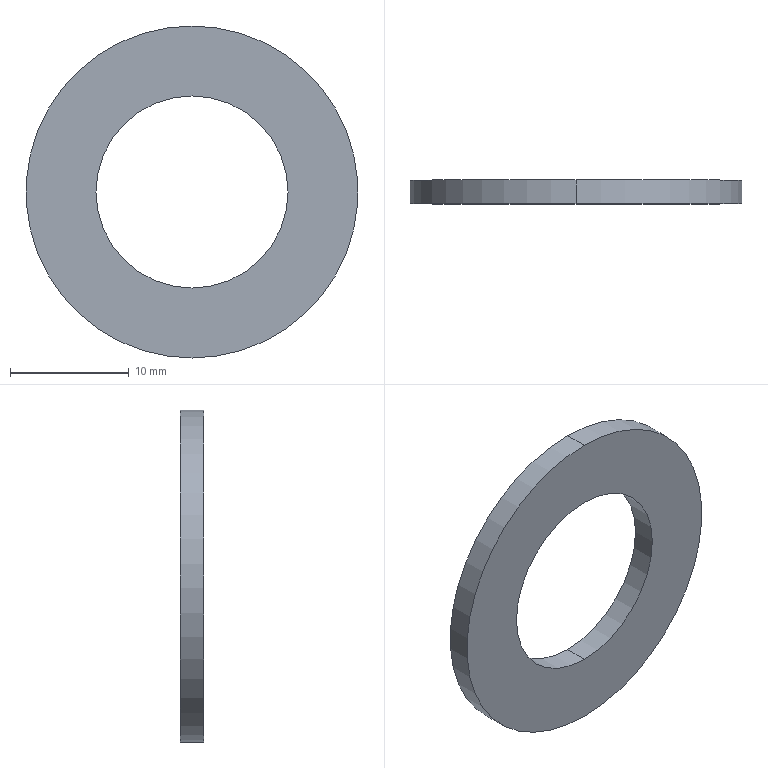Part | STEP file | PN_0004 Spring seat | 1 solid | 6 faces | box 28 x 2 x 28 mm | volume 819.265 mm3 | cylinder 4 | plane 2 | commonest cylinder face diameters 16.2 x2 28 x2
STEP:
#1=CARTESIAN_POINT('',(0.,0.,0.));
#2=DIRECTION('',(0.,0.,1.));
#3=DIRECTION('',(1.,0.,0.));
#4=AXIS2_PLACEMENT_3D('',#1,#2,#3);
#5=CARTESIAN_POINT('',(0.,2.,-8.1));
#6=VERTEX_POINT('',#5);
#7=CARTESIAN_POINT('',(0.,0.,-8.1));
#8=VERTEX_POINT('',#7);
#9=CARTESIAN_POINT('',(0.,2.,-8.1));
#10=DIRECTION('',(0.,-1.,0.));
#11=VECTOR('',#10,1.);
#12=LINE('',#9,#11);
#13=CARTESIAN_POINT('',(0.,2.,0.));
#14=DIRECTION('',(0.,-1.,0.));
#15=DIRECTION('',(0.,0.,-1.));
#16=AXIS2_PLACEMENT_3D('',#13,#14,#15);
#17=CYLINDRICAL_SURFACE('',#16,8.1);
#18=CARTESIAN_POINT('',(6.283,0.));
#19=DIRECTION('',(0.,1.));
#20=VECTOR('',#19,1.);
#21=LINE('',#18,#20);
#22=(GEOMETRIC_REPRESENTATION_CONTEXT(2)PARAMETRIC_REPRESENTATION_CONTEXT()REPRESENTATION_CONTEXT('',''));
#23=DEFINITIONAL_REPRESENTATION('',(#21),#22);
#24=PCURVE('',#17,#23);
#25=CARTESIAN_POINT('',(0.,2.,0.));
#26=DIRECTION('',(0.,-1.,0.));
#27=DIRECTION('',(0.,0.,-1.));
#28=AXIS2_PLACEMENT_3D('',#25,#26,#27);
#29=CYLINDRICAL_SURFACE('',#28,8.1);
#30=CARTESIAN_POINT('',(0.,0.));
#31=DIRECTION('',(0.,1.));
#32=VECTOR('',#31,1.);
#33=LINE('',#30,#32);
#34=(GEOMETRIC_REPRESENTATION_CONTEXT(2)PARAMETRIC_REPRESENTATION_CONTEXT()REPRESENTATION_CONTEXT('',''));
#35=DEFINITIONAL_REPRESENTATION('',(#33),#34);
#36=PCURVE('',#29,#35);
#37=SURFACE_CURVE('',#12,(#24,#36),.PCURVE_S1.);
#38=EDGE_CURVE('',#6,#8,#37,.T.);
#39=ORIENTED_EDGE('',*,*,#38,.T.);
#40=CARTESIAN_POINT('',(0.,0.,8.1));
#41=VERTEX_POINT('',#40);
#42=CARTESIAN_POINT('',(0.,0.,0.));
#43=DIRECTION('',(0.,1.,0.));
#44=DIRECTION('',(0.,0.,-1.));
#45=AXIS2_PLACEMENT_3D('',#42,#43,#44);
#46=CIRCLE('',#45,8.1);
#47=CARTESIAN_POINT('',(6.283,2.));
#48=DIRECTION('',(-1.,0.));
#49=VECTOR('',#48,1.);
#50=LINE('',#47,#49);
#51=(GEOMETRIC_REPRESENTATION_CONTEXT(2)PARAMETRIC_REPRESENTATION_CONTEXT()REPRESENTATION_CONTEXT('',''));
#52=DEFINITIONAL_REPRESENTATION('',(#50),#51);
#53=PCURVE('',#17,#52);
#54=CARTESIAN_POINT('',(0.,0.,0.));
#55=DIRECTION('',(0.,1.,0.));
#56=DIRECTION('',(0.,0.,1.));
#57=AXIS2_PLACEMENT_3D('',#54,#55,#56);
#58=PLANE('',#57);
#59=CARTESIAN_POINT('',(0.,0.));
#60=DIRECTION('',(-1.,0.));
#61=AXIS2_PLACEMENT_2D('',#59,#60);
#62=CIRCLE('',#61,8.1);
#63=(GEOMETRIC_REPRESENTATION_CONTEXT(2)PARAMETRIC_REPRESENTATION_CONTEXT()REPRESENTATION_CONTEXT('',''));
#64=DEFINITIONAL_REPRESENTATION('',(#62),#63);
#65=PCURVE('',#58,#64);
#66=SURFACE_CURVE('',#46,(#53,#65),.PCURVE_S1.);
#67=EDGE_CURVE('',#8,#41,#66,.T.);
#68=ORIENTED_EDGE('',*,*,#67,.T.);
#69=CARTESIAN_POINT('',(0.,2.,8.1));
#70=VERTEX_POINT('',#69);
#71=CARTESIAN_POINT('',(0.,2.,8.1));
#72=DIRECTION('',(0.,-1.,0.));
#73=VECTOR('',#72,1.);
#74=LINE('',#71,#73);
#75=CARTESIAN_POINT('',(3.142,0.));
#76=DIRECTION('',(0.,1.));
#77=VECTOR('',#76,1.);
#78=LINE('',#75,#77);
#79=(GEOMETRIC_REPRESENTATION_CONTEXT(2)PARAMETRIC_REPRESENTATION_CONTEXT()REPRESENTATION_CONTEXT('',''));
#80=DEFINITIONAL_REPRESENTATION('',(#78),#79);
#81=PCURVE('',#17,#80);
#82=CARTESIAN_POINT('',(3.142,0.));
#83=DIRECTION('',(0.,1.));
#84=VECTOR('',#83,1.);
#85=LINE('',#82,#84);
#86=(GEOMETRIC_REPRESENTATION_CONTEXT(2)PARAMETRIC_REPRESENTATION_CONTEXT()REPRESENTATION_CONTEXT('',''));
#87=DEFINITIONAL_REPRESENTATION('',(#85),#86);
#88=PCURVE('',#29,#87);
#89=SURFACE_CURVE('',#74,(#81,#88),.PCURVE_S1.);
#90=EDGE_CURVE('',#70,#41,#89,.T.);
#91=ORIENTED_EDGE('',*,*,#90,.F.);
#92=CARTESIAN_POINT('',(0.,2.,0.));
#93=DIRECTION('',(0.,-1.,0.));
#94=DIRECTION('',(0.,0.,-1.));
#95=AXIS2_PLACEMENT_3D('',#92,#93,#94);
#96=CIRCLE('',#95,8.1);
#97=CARTESIAN_POINT('',(0.,0.));
#98=DIRECTION('',(1.,0.));
#99=VECTOR('',#98,1.);
#100=LINE('',#97,#99);
#101=(GEOMETRIC_REPRESENTATION_CONTEXT(2)PARAMETRIC_REPRESENTATION_CONTEXT()REPRESENTATION_CONTEXT('',''));
#102=DEFINITIONAL_REPRESENTATION('',(#100),#101);
#103=PCURVE('',#17,#102);
#104=CARTESIAN_POINT('',(0.,2.,0.));
#105=DIRECTION('',(0.,1.,0.));
#106=DIRECTION('',(0.,0.,1.));
#107=AXIS2_PLACEMENT_3D('',#104,#105,#106);
#108=PLANE('',#107);
#109=CARTESIAN_POINT('',(-8.1,0.));
#110=CARTESIAN_POINT('',(-8.1,14.03));
#111=CARTESIAN_POINT('',(4.05,7.015));
#112=CARTESIAN_POINT('',(16.2,0.));
#113=CARTESIAN_POINT('',(4.05,-7.015));
#114=CARTESIAN_POINT('',(-8.1,-14.03));
#115=CARTESIAN_POINT('',(-8.1,0.));
#116=(BOUNDED_CURVE()B_SPLINE_CURVE(2,(#109,#110,#111,#112,#113,#114,#115),.UNSPECIFIED.,.T.,.F.)B_SPLINE_CURVE_WITH_KNOTS((1,2,2,2,2,1),(-2.094,0.,2.094,4.189,6.283,8.378),.UNSPECIFIED.)CURVE()GEOMETRIC_REPRESENTATION_ITEM()RATIONAL_B_SPLINE_CURVE((1.,0.5,1.,0.5,1.,0.5,1.))REPRESENTATION_ITEM(''));
#117=(GEOMETRIC_REPRESENTATION_CONTEXT(2)PARAMETRIC_REPRESENTATION_CONTEXT()REPRESENTATION_CONTEXT('',''));
#118=DEFINITIONAL_REPRESENTATION('',(#116),#117);
#119=PCURVE('',#108,#118);
#120=SURFACE_CURVE('',#96,(#103,#119),.PCURVE_S1.);
#121=EDGE_CURVE('',#70,#6,#120,.T.);
#122=ORIENTED_EDGE('',*,*,#121,.T.);
#123=EDGE_LOOP('',(#39,#68,#91,#122));
#124=FACE_BOUND('',#123,.F.);
#125=ADVANCED_FACE('',(#124),#17,.F.);
#126=CARTESIAN_POINT('',(0.,2.,14.));
#127=VERTEX_POINT('',#126);
#128=CARTESIAN_POINT('',(0.,2.,-14.));
#129=VERTEX_POINT('',#128);
#130=CARTESIAN_POINT('',(0.,2.,0.));
#131=DIRECTION('',(0.,1.,0.));
#132=DIRECTION('',(0.,0.,-1.));
#133=AXIS2_PLACEMENT_3D('',#130,#131,#132);
#134=CIRCLE('',#133,14.);
#135=CARTESIAN_POINT('',(0.,2.,0.));
#136=DIRECTION('',(0.,-1.,0.));
#137=DIRECTION('',(0.,0.,-1.));
#138=AXIS2_PLACEMENT_3D('',#135,#136,#137);
#139=CYLINDRICAL_SURFACE('',#138,14.);
#140=CARTESIAN_POINT('',(6.283,0.));
#141=DIRECTION('',(-1.,0.));
#142=VECTOR('',#141,1.);
#143=LINE('',#140,#142);
#144=(GEOMETRIC_REPRESENTATION_CONTEXT(2)PARAMETRIC_REPRESENTATION_CONTEXT()REPRESENTATION_CONTEXT('',''));
#145=DEFINITIONAL_REPRESENTATION('',(#143),#144);
#146=PCURVE('',#139,#145);
#147=CARTESIAN_POINT('',(0.,0.));
#148=DIRECTION('',(-1.,0.));
#149=AXIS2_PLACEMENT_2D('',#147,#148);
#150=CIRCLE('',#149,14.);
#151=(GEOMETRIC_REPRESENTATION_CONTEXT(2)PARAMETRIC_REPRESENTATION_CONTEXT()REPRESENTATION_CONTEXT('',''));
#152=DEFINITIONAL_REPRESENTATION('',(#150),#151);
#153=PCURVE('',#108,#152);
#154=SURFACE_CURVE('',#134,(#146,#153),.PCURVE_S1.);
#155=EDGE_CURVE('',#127,#129,#154,.T.);
#156=ORIENTED_EDGE('',*,*,#155,.F.);
#157=CARTESIAN_POINT('',(0.,0.,14.));
#158=VERTEX_POINT('',#157);
#159=CARTESIAN_POINT('',(0.,2.,14.));
#160=DIRECTION('',(0.,-1.,0.));
#161=VECTOR('',#160,1.);
#162=LINE('',#159,#161);
#163=CARTESIAN_POINT('',(3.142,0.));
#164=DIRECTION('',(0.,1.));
#165=VECTOR('',#164,1.);
#166=LINE('',#163,#165);
#167=(GEOMETRIC_REPRESENTATION_CONTEXT(2)PARAMETRIC_REPRESENTATION_CONTEXT()REPRESENTATION_CONTEXT('',''));
#168=DEFINITIONAL_REPRESENTATION('',(#166),#167);
#169=PCURVE('',#139,#168);
#170=CARTESIAN_POINT('',(0.,2.,0.));
#171=DIRECTION('',(0.,-1.,0.));
#172=DIRECTION('',(0.,0.,-1.));
#173=AXIS2_PLACEMENT_3D('',#170,#171,#172);
#174=CYLINDRICAL_SURFACE('',#173,14.);
#175=CARTESIAN_POINT('',(3.142,0.));
#176=DIRECTION('',(0.,1.));
#177=VECTOR('',#176,1.);
#178=LINE('',#175,#177);
#179=(GEOMETRIC_REPRESENTATION_CONTEXT(2)PARAMETRIC_REPRESENTATION_CONTEXT()REPRESENTATION_CONTEXT('',''));
#180=DEFINITIONAL_REPRESENTATION('',(#178),#179);
#181=PCURVE('',#174,#180);
#182=SURFACE_CURVE('',#162,(#169,#181),.PCURVE_S1.);
#183=EDGE_CURVE('',#127,#158,#182,.T.);
#184=ORIENTED_EDGE('',*,*,#183,.T.);
#185=CARTESIAN_POINT('',(0.,0.,-14.));
#186=VERTEX_POINT('',#185);
#187=CARTESIAN_POINT('',(0.,0.,0.));
#188=DIRECTION('',(0.,1.,0.));
#189=DIRECTION('',(0.,0.,-1.));
#190=AXIS2_PLACEMENT_3D('',#187,#188,#189);
#191=CIRCLE('',#190,14.);
#192=CARTESIAN_POINT('',(6.283,2.));
#193=DIRECTION('',(-1.,0.));
#194=VECTOR('',#193,1.);
#195=LINE('',#192,#194);
#196=(GEOMETRIC_REPRESENTATION_CONTEXT(2)PARAMETRIC_REPRESENTATION_CONTEXT()REPRESENTATION_CONTEXT('',''));
#197=DEFINITIONAL_REPRESENTATION('',(#195),#196);
#198=PCURVE('',#139,#197);
#199=CARTESIAN_POINT('',(0.,0.));
#200=DIRECTION('',(-1.,0.));
#201=AXIS2_PLACEMENT_2D('',#199,#200);
#202=CIRCLE('',#201,14.);
#203=(GEOMETRIC_REPRESENTATION_CONTEXT(2)PARAMETRIC_REPRESENTATION_CONTEXT()REPRESENTATION_CONTEXT('',''));
#204=DEFINITIONAL_REPRESENTATION('',(#202),#203);
#205=PCURVE('',#58,#204);
#206=SURFACE_CURVE('',#191,(#198,#205),.PCURVE_S1.);
#207=EDGE_CURVE('',#158,#186,#206,.T.);
#208=ORIENTED_EDGE('',*,*,#207,.T.);
#209=CARTESIAN_POINT('',(0.,2.,-14.));
#210=DIRECTION('',(0.,-1.,0.));
#211=VECTOR('',#210,1.);
#212=LINE('',#209,#211);
#213=CARTESIAN_POINT('',(0.,0.));
#214=DIRECTION('',(0.,1.));
#215=VECTOR('',#214,1.);
#216=LINE('',#213,#215);
#217=(GEOMETRIC_REPRESENTATION_CONTEXT(2)PARAMETRIC_REPRESENTATION_CONTEXT()REPRESENTATION_CONTEXT('',''));
#218=DEFINITIONAL_REPRESENTATION('',(#216),#217);
#219=PCURVE('',#139,#218);
#220=CARTESIAN_POINT('',(6.283,0.));
#221=DIRECTION('',(0.,1.));
#222=VECTOR('',#221,1.);
#223=LINE('',#220,#222);
#224=(GEOMETRIC_REPRESENTATION_CONTEXT(2)PARAMETRIC_REPRESENTATION_CONTEXT()REPRESENTATION_CONTEXT('',''));
#225=DEFINITIONAL_REPRESENTATION('',(#223),#224);
#226=PCURVE('',#174,#225);
#227=SURFACE_CURVE('',#212,(#219,#226),.PCURVE_S1.);
#228=EDGE_CURVE('',#129,#186,#227,.T.);
#229=ORIENTED_EDGE('',*,*,#228,.F.);
#230=EDGE_LOOP('',(#156,#184,#208,#229));
#231=FACE_BOUND('',#230,.T.);
#232=ADVANCED_FACE('',(#231),#139,.T.);
#233=CARTESIAN_POINT('',(0.,2.,0.));
#234=DIRECTION('',(0.,-1.,0.));
#235=DIRECTION('',(0.,0.,-1.));
#236=AXIS2_PLACEMENT_3D('',#233,#234,#235);
#237=CIRCLE('',#236,8.1);
#238=CARTESIAN_POINT('',(-8.1,0.));
#239=CARTESIAN_POINT('',(-8.1,14.03));
#240=CARTESIAN_POINT('',(4.05,7.015));
#241=CARTESIAN_POINT('',(16.2,0.));
#242=CARTESIAN_POINT('',(4.05,-7.015));
#243=CARTESIAN_POINT('',(-8.1,-14.03));
#244=CARTESIAN_POINT('',(-8.1,0.));
#245=(BOUNDED_CURVE()B_SPLINE_CURVE(2,(#238,#239,#240,#241,#242,#243,#244),.UNSPECIFIED.,.T.,.F.)B_SPLINE_CURVE_WITH_KNOTS((1,2,2,2,2,1),(-2.094,0.,2.094,4.189,6.283,8.378),.UNSPECIFIED.)CURVE()GEOMETRIC_REPRESENTATION_ITEM()RATIONAL_B_SPLINE_CURVE((1.,0.5,1.,0.5,1.,0.5,1.))REPRESENTATION_ITEM(''));
#246=(GEOMETRIC_REPRESENTATION_CONTEXT(2)PARAMETRIC_REPRESENTATION_CONTEXT()REPRESENTATION_CONTEXT('',''));
#247=DEFINITIONAL_REPRESENTATION('',(#245),#246);
#248=PCURVE('',#108,#247);
#249=CARTESIAN_POINT('',(0.,0.));
#250=DIRECTION('',(1.,0.));
#251=VECTOR('',#250,1.);
#252=LINE('',#249,#251);
#253=(GEOMETRIC_REPRESENTATION_CONTEXT(2)PARAMETRIC_REPRESENTATION_CONTEXT()REPRESENTATION_CONTEXT('',''));
#254=DEFINITIONAL_REPRESENTATION('',(#252),#253);
#255=PCURVE('',#29,#254);
#256=SURFACE_CURVE('',#237,(#248,#255),.PCURVE_S1.);
#257=EDGE_CURVE('',#6,#70,#256,.T.);
#258=ORIENTED_EDGE('',*,*,#257,.T.);
#259=ORIENTED_EDGE('',*,*,#121,.T.);
#260=EDGE_LOOP('',(#258,#259));
#261=FACE_BOUND('',#260,.T.);
#262=CARTESIAN_POINT('',(0.,2.,0.));
#263=DIRECTION('',(0.,1.,0.));
#264=DIRECTION('',(0.,0.,-1.));
#265=AXIS2_PLACEMENT_3D('',#262,#263,#264);
#266=CIRCLE('',#265,14.);
#267=CARTESIAN_POINT('',(0.,0.));
#268=DIRECTION('',(-1.,0.));
#269=AXIS2_PLACEMENT_2D('',#267,#268);
#270=CIRCLE('',#269,14.);
#271=(GEOMETRIC_REPRESENTATION_CONTEXT(2)PARAMETRIC_REPRESENTATION_CONTEXT()REPRESENTATION_CONTEXT('',''));
#272=DEFINITIONAL_REPRESENTATION('',(#270),#271);
#273=PCURVE('',#108,#272);
#274=CARTESIAN_POINT('',(6.283,0.));
#275=DIRECTION('',(-1.,0.));
#276=VECTOR('',#275,1.);
#277=LINE('',#274,#276);
#278=(GEOMETRIC_REPRESENTATION_CONTEXT(2)PARAMETRIC_REPRESENTATION_CONTEXT()REPRESENTATION_CONTEXT('',''));
#279=DEFINITIONAL_REPRESENTATION('',(#277),#278);
#280=PCURVE('',#174,#279);
#281=SURFACE_CURVE('',#266,(#273,#280),.PCURVE_S1.);
#282=EDGE_CURVE('',#129,#127,#281,.T.);
#283=ORIENTED_EDGE('',*,*,#282,.T.);
#284=ORIENTED_EDGE('',*,*,#155,.T.);
#285=EDGE_LOOP('',(#283,#284));
#286=FACE_BOUND('',#285,.T.);
#287=ADVANCED_FACE('',(#261,#286),#108,.T.);
#288=CARTESIAN_POINT('',(0.,0.,0.));
#289=DIRECTION('',(0.,1.,0.));
#290=DIRECTION('',(0.,0.,-1.));
#291=AXIS2_PLACEMENT_3D('',#288,#289,#290);
#292=CIRCLE('',#291,8.1);
#293=CARTESIAN_POINT('',(6.283,2.));
#294=DIRECTION('',(-1.,0.));
#295=VECTOR('',#294,1.);
#296=LINE('',#293,#295);
#297=(GEOMETRIC_REPRESENTATION_CONTEXT(2)PARAMETRIC_REPRESENTATION_CONTEXT()REPRESENTATION_CONTEXT('',''));
#298=DEFINITIONAL_REPRESENTATION('',(#296),#297);
#299=PCURVE('',#29,#298);
#300=CARTESIAN_POINT('',(0.,0.));
#301=DIRECTION('',(-1.,0.));
#302=AXIS2_PLACEMENT_2D('',#300,#301);
#303=CIRCLE('',#302,8.1);
#304=(GEOMETRIC_REPRESENTATION_CONTEXT(2)PARAMETRIC_REPRESENTATION_CONTEXT()REPRESENTATION_CONTEXT('',''));
#305=DEFINITIONAL_REPRESENTATION('',(#303),#304);
#306=PCURVE('',#58,#305);
#307=SURFACE_CURVE('',#292,(#299,#306),.PCURVE_S1.);
#308=EDGE_CURVE('',#41,#8,#307,.T.);
#309=ORIENTED_EDGE('',*,*,#308,.T.);
#310=ORIENTED_EDGE('',*,*,#38,.F.);
#311=ORIENTED_EDGE('',*,*,#257,.T.);
#312=ORIENTED_EDGE('',*,*,#90,.T.);
#313=EDGE_LOOP('',(#309,#310,#311,#312));
#314=FACE_BOUND('',#313,.F.);
#315=ADVANCED_FACE('',(#314),#29,.F.);
#316=ORIENTED_EDGE('',*,*,#183,.F.);
#317=ORIENTED_EDGE('',*,*,#282,.F.);
#318=ORIENTED_EDGE('',*,*,#228,.T.);
#319=CARTESIAN_POINT('',(0.,0.,0.));
#320=DIRECTION('',(0.,1.,0.));
#321=DIRECTION('',(0.,0.,-1.));
#322=AXIS2_PLACEMENT_3D('',#319,#320,#321);
#323=CIRCLE('',#322,14.);
#324=CARTESIAN_POINT('',(6.283,2.));
#325=DIRECTION('',(-1.,0.));
#326=VECTOR('',#325,1.);
#327=LINE('',#324,#326);
#328=(GEOMETRIC_REPRESENTATION_CONTEXT(2)PARAMETRIC_REPRESENTATION_CONTEXT()REPRESENTATION_CONTEXT('',''));
#329=DEFINITIONAL_REPRESENTATION('',(#327),#328);
#330=PCURVE('',#174,#329);
#331=CARTESIAN_POINT('',(0.,0.));
#332=DIRECTION('',(-1.,0.));
#333=AXIS2_PLACEMENT_2D('',#331,#332);
#334=CIRCLE('',#333,14.);
#335=(GEOMETRIC_REPRESENTATION_CONTEXT(2)PARAMETRIC_REPRESENTATION_CONTEXT()REPRESENTATION_CONTEXT('',''));
#336=DEFINITIONAL_REPRESENTATION('',(#334),#335);
#337=PCURVE('',#58,#336);
#338=SURFACE_CURVE('',#323,(#330,#337),.PCURVE_S1.);
#339=EDGE_CURVE('',#186,#158,#338,.T.);
#340=ORIENTED_EDGE('',*,*,#339,.T.);
#341=EDGE_LOOP('',(#316,#317,#318,#340));
#342=FACE_BOUND('',#341,.T.);
#343=ADVANCED_FACE('',(#342),#174,.T.);
#344=ORIENTED_EDGE('',*,*,#67,.T.);
#345=ORIENTED_EDGE('',*,*,#308,.T.);
#346=EDGE_LOOP('',(#344,#345));
#347=FACE_BOUND('',#346,.T.);
#348=ORIENTED_EDGE('',*,*,#339,.F.);
#349=ORIENTED_EDGE('',*,*,#207,.F.);
#350=EDGE_LOOP('',(#348,#349));
#351=FACE_BOUND('',#350,.T.);
#352=ADVANCED_FACE('',(#347,#351),#58,.F.);
#353=CLOSED_SHELL('',(#125,#232,#287,#315,#343,#352));
#354=MANIFOLD_SOLID_BREP('',#353);
#355=(LENGTH_UNIT()NAMED_UNIT(*)SI_UNIT(.MILLI.,.METRE.));
#356=UNCERTAINTY_MEASURE_WITH_UNIT(LENGTH_MEASURE(0.0000001),#355,'','');
#357=(NAMED_UNIT(*)PLANE_ANGLE_UNIT()SI_UNIT($,.RADIAN.));
#358=(NAMED_UNIT(*)SI_UNIT($,.STERADIAN.)SOLID_ANGLE_UNIT());
#359=(GEOMETRIC_REPRESENTATION_CONTEXT(3)GLOBAL_UNCERTAINTY_ASSIGNED_CONTEXT((#356))GLOBAL_UNIT_ASSIGNED_CONTEXT((#355,#357,#358))REPRESENTATION_CONTEXT('',''));
#360=ADVANCED_BREP_SHAPE_REPRESENTATION('',(#4,#354),#359);